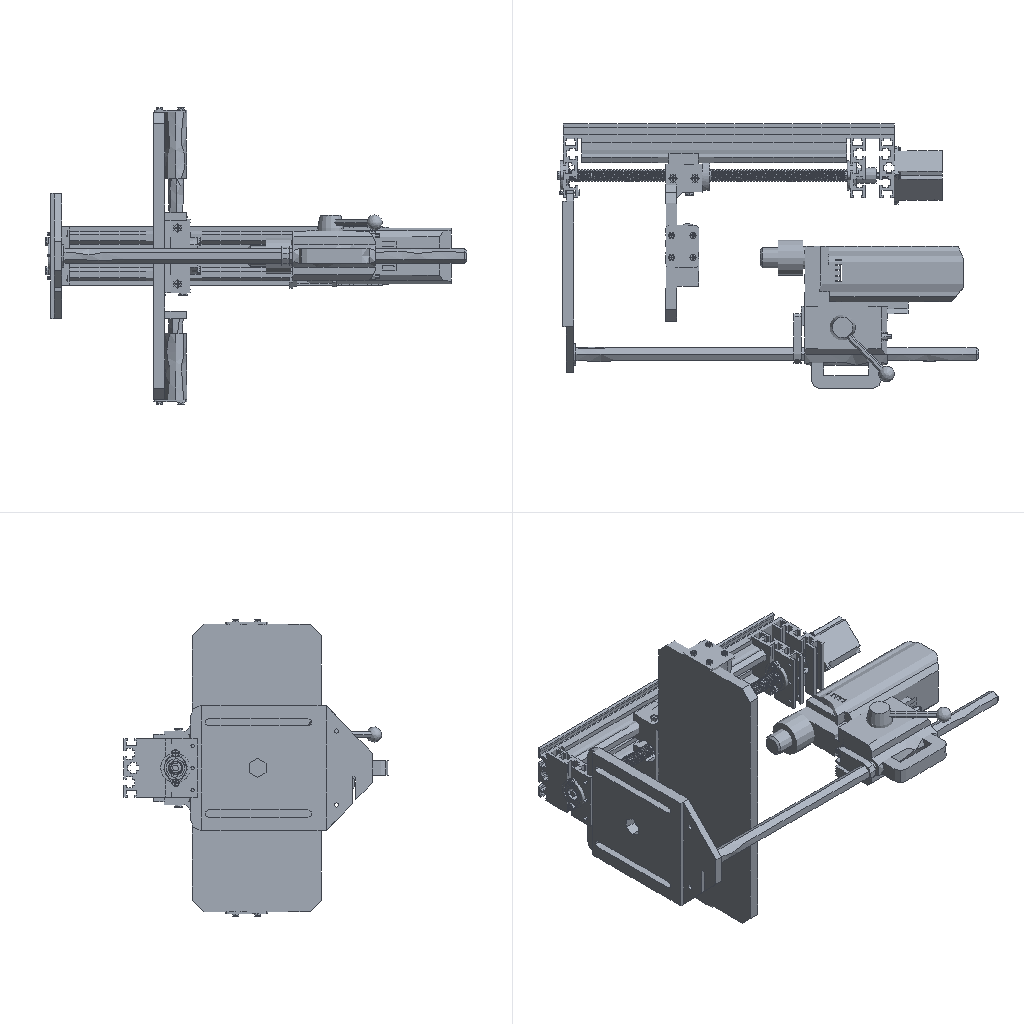Simulation study | ansys workbench
Set-up summary:
category,name,step,type,value,unit,region
solver,ansys_workbench
units,mm-N-s-tonne (MPa),,stated,"/units,MPA"
analysis,LS1,,static
load_step,LS1,LS1,static,nsubst=1; time=1
mesh,nodes,,,176175
mesh,elements,,,123008
element_type,SOLID187,,,82523
element_type,TARGE170,,,19068
element_type,CONTA174,,,19068
element_type,SOLID186,,,1937
element_type,SURF154,,,412
material,Structural Steel,,E,200000,tonne s^-2 mm^-1
material,Structural Steel,,nu,0.3
material,Structural Steel,,density,7.85e-09,tonne mm^-3
material,Structural Steel,,conductivity,60.5,tonne mm s^-3 C^-1
material,Structural Steel,,specific_heat,4.34e+08,mm^2 s^-2 C^-1
material,Structural Steel,,cte,1.2e-05,C^-1
material,Structural Steel,,permeability,10000
material,Structural Steel,,resistivity,0.00017,ohm mm
load,Define Force Using Surface Effect Elements,LS1,surface-effect pres face 1,-0.05982,,SURF154 #299
load,Define Force Using Surface Effect Elements,LS1,surface-effect pres face 3,-0.1976,,SURF154 #300
load,Define Force Using Surface Effect Elements,LS1,surface-effect pres face 3,0.1976,,SURF154 #301
bc,Fixed Supports,model,fixed,[dofs=ALL],,_FIXEDSU
contact,Contact Region,,bonded (always),element=CONTA174
contact,Contact Region 2,,bonded (always),element=CONTA174
contact,Contact Region 3,,bonded (always),element=CONTA174
contact,Contact Region 4,,bonded (always),element=CONTA174
contact,Contact Region 5,,bonded (always),element=CONTA174
contact,Contact Region 6,,bonded (always),element=CONTA174
contact,Contact Region 7,,bonded (always),element=CONTA174
contact,Contact Region 8,,bonded (always),element=CONTA174
contact,Contact Region 9,,bonded (always),element=CONTA174
contact,Contact Region 10,,bonded (always),element=CONTA174
contact,Contact Region 11,,bonded (always),element=CONTA174
contact,Contact Region 12,,bonded (always),element=CONTA174
contact,Contact Region 13,,bonded (always),element=CONTA174
contact,Contact Region 14,,bonded (always),element=CONTA174
contact,Contact Region 15,,bonded (always),element=CONTA174
contact,Contact Region 16,,bonded (always),element=CONTA174
contact,Contact Region 17,,bonded (always),element=CONTA174
contact,Contact Region 18,,bonded (always),element=CONTA174
contact,Contact Region 19,,bonded (always),element=CONTA174
contact,Contact Region 20,,bonded (always),element=CONTA174
contact,Contact Region 21,,bonded (always),element=CONTA174
contact,Contact Region 22,,bonded (always),element=CONTA174
contact,Contact Region 23,,bonded (always),element=CONTA174
contact,Contact Region 24,,bonded (always),element=CONTA174
contact,Contact Region 25,,bonded (always),element=CONTA174
contact,Contact Region 26,,bonded (always),element=CONTA174
contact,Contact Region 27,,bonded (always),element=CONTA174
contact,Contact Region 28,,bonded (always),element=CONTA174
contact,Contact Region 29,,bonded (always),element=CONTA174
contact,Contact Region 30,,bonded (always),element=CONTA174
contact,Contact Region 31,,bonded (always),element=CONTA174
contact,Contact Region 32,,bonded (always),element=CONTA174
contact,Contact Region 33,,bonded (always),element=CONTA174
contact,Contact Region 34,,bonded (always),element=CONTA174
contact,Contact Region 35,,bonded (always),element=CONTA174
contact,Contact Region 36,,bonded (always),element=CONTA174
contact,Contact Region 37,,bonded (always),element=CONTA174
contact,Contact Region 38,,bonded (always),element=CONTA174
contact,Contact Region 39,,bonded (always),element=CONTA174
contact,Contact Region 40,,bonded (always),element=CONTA174
contact,Contact Region 41,,bonded (always),element=CONTA174
contact,Contact Region 42,,bonded (always),element=CONTA174
contact,Contact Region 43,,bonded (always),element=CONTA174
contact,Contact Region 44,,bonded (always),element=CONTA174
contact,Contact Region 45,,bonded (always),element=CONTA174
contact,Contact Region 46,,bonded (always),element=CONTA174
contact,Contact Region 47,,bonded (always),element=CONTA174
contact,Contact Region 48,,bonded (always),element=CONTA174
contact,Contact Region 49,,bonded (always),element=CONTA174
contact,Contact Region 50,,bonded (always),element=CONTA174
contact,Contact Region 51,,bonded (always),element=CONTA174
contact,Contact Region 52,,bonded (always),element=CONTA174
contact,Contact Region 53,,bonded (always),element=CONTA174
contact,Contact Region 54,,bonded (always),element=CONTA174
contact,Contact Region 55,,bonded (always),element=CONTA174
contact,Contact Region 56,,bonded (always),element=CONTA174
contact,Contact Region 57,,bonded (always),element=CONTA174
contact,Contact Region 58,,bonded (always),element=CONTA174
contact,Contact Region 59,,bonded (always),element=CONTA174
contact,Contact Region 60,,bonded (always),element=CONTA174
contact,Contact Region 61,,bonded (always),element=CONTA174
contact,Contact Region 62,,bonded (always),element=CONTA174
contact,Contact Region 63,,bonded (always),element=CONTA174
contact,Contact Region 64,,bonded (always),element=CONTA174
contact,Contact Region 65,,bonded (always),element=CONTA174
contact,Contact Region 66,,bonded (always),element=CONTA174
contact,Contact Region 67,,bonded (always),element=CONTA174
contact,Contact Region 68,,bonded (always),element=CONTA174
contact,Contact Region 69,,bonded (always),element=CONTA174
contact,Contact Region 70,,bonded (always),element=CONTA174
contact,Contact Region 71,,bonded (always),element=CONTA174
contact,Contact Region 72,,bonded (always),element=CONTA174
contact,Contact Region 73,,bonded (always),element=CONTA174
contact,Contact Region 74,,bonded (always),element=CONTA174
contact,Contact Region 75,,bonded (always),element=CONTA174
contact,Contact Region 76,,bonded (always),element=CONTA174
contact,Contact Region 77,,bonded (always),element=CONTA174
contact,Contact Region 78,,bonded (always),element=CONTA174
contact,Contact Region 79,,bonded (always),element=CONTA174
contact,Contact Region 80,,bonded (always),element=CONTA174
contact,Contact Region 81,,bonded (always),element=CONTA174
contact,Contact Region 82,,bonded (always),element=CONTA174
contact,Contact Region 83,,bonded (always),element=CONTA174
contact,Contact Region 84,,bonded (always),element=CONTA174
contact,Contact Region 85,,bonded (always),element=CONTA174
contact,Contact Region 86,,bonded (always),element=CONTA174
contact,Contact Region 87,,bonded (always),element=CONTA174
contact,Contact Region 88,,bonded (always),element=CONTA174
contact,Contact Region 89,,bonded (always),element=CONTA174
contact,Contact Region 90,,bonded (always),element=CONTA174
contact,Contact Region 91,,bonded (always),element=CONTA174
contact,Contact Region 92,,bonded (always),element=CONTA174
contact,Contact Region 93,,bonded (always),element=CONTA174
contact,Contact Region 94,,bonded (always),element=CONTA174
contact,Contact Region 95,,bonded (always),element=CONTA174
contact,Contact Region 96,,bonded (always),element=CONTA174
contact,Contact Region 97,,bonded (always),element=CONTA174
contact,Contact Region 98,,bonded (always),element=CONTA174
contact,Contact Region 99,,bonded (always),element=CONTA174
contact,Contact Region 100,,bonded (always),element=CONTA174
contact,Contact Region 101,,bonded (always),element=CONTA174
contact,Contact Region 102,,bonded (always),element=CONTA174
contact,Contact Region 103,,bonded (always),element=CONTA174
contact,Contact Region 104,,bonded (always),element=CONTA174
contact,Contact Region 105,,bonded (always),element=CONTA174
contact,Contact Region 106,,bonded (always),element=CONTA174
contact,Contact Region 107,,bonded (always),element=CONTA174
contact,Contact Region 108,,bonded (always),element=CONTA174
contact,Contact Region 109,,bonded (always),element=CONTA174
contact,Contact Region 110,,bonded (always),element=CONTA174
contact,Contact Region 111,,bonded (always),element=CONTA174
contact,Contact Region 112,,bonded (always),element=CONTA174
named_set,_FIXEDSU,,node,69000
Ansys APDL input file, long lists of numbers shortened:
/batch
/config,noeldb,1     ! force off writing results to database
*get,_wallstrt,active,,time,wall
! ANSYS input file written by Workbench version 2022 R1
! File used for geometry attach:
/title,wbnew--____ (B5)
! ****** Begin Custom Load Command Snippet ******
/COM, ACT Extensions:
/COM,     LSDYNA, 2021.1
/COM,
! ****** End   Custom Load Command Snippet ******
*DIM,_wb_ProjectScratch_dir,string,248
_wb_ProjectScratch_dir(1) = ''
*DIM,_wb_SolverFiles_dir,string,248
_wb_SolverFiles_dir(1) = ''
*DIM,_wb_userfiles_dir,string,248
_wb_userfiles_dir(1) = ''
/com,--- Data in consistent NMM units. See Solving Units in the help system for more information.
/units,MPA
/nopr
/wb,file,start              !  signify a WB generated input file
/prep7
! Turn off shape checking because checks already performed inside WB mesher.
! See help system for more information.
SHPP,OFF,,NOWARN
/nolist
etcon,set             ! allow ANSYS to choose best KEYOP's for 180x elements, resets any applicable keyopt to MAPDL defaults
/com,*********** Nodes for the whole assembly ***********
nblock,3,,193792
(1i9,3e20.9e3)
        1     4.544231993E+01    -1.675656162E+02     8.308123616E-01
! (176174 more lines like these left out)
-1
/wb,elem,start            !  set before creation of elements
/com,*********** Elements for Body 1 "____|__-__3" ***********
et,1,187
eblock,19,solid,,10209
(19i9)
        1        1        1        1        0        0        0        0       10        0    47846    97468   101014    97470    97469   101844   101853   101839   101838
! (20417 more lines like these left out)
-1
/com,*********** Elements for Body 2 "____|__-__5" ***********
et,2,187
eblock,19,solid,,2459
(19i9)
        2        2        2        2        0        0        0        0       10        0    60222   123346   123792   124169   124165   124991   127779   124995   124994
! (4917 more lines like these left out)
-1
/com,*********** Elements for Body 3 "____|__-__5[2]" ***********
et,3,187
eblock,19,solid,,2459
(19i9)
        3        3        3        3        0        0        0        0       10        0    64453   133020   133466   133843   133839   134665   137453   134669   134668
! (4917 more lines like these left out)
-1
/com,*********** Elements for Body 4 "____ 2|__-__5" ***********
et,4,187
eblock,19,solid,,1587
(19i9)
        4        4        4        4        0        0        0        0       10        0    67164   139805   140360   139811   139812   140972   140997   140969   140970
! (3173 more lines like these left out)
-1
/com,*********** Elements for Body 5 "_______|__-__4" ***********
et,5,186
keyo,5,2,1          ! set full integration on SOLID186
eblock,19,solid,,252
(19i9)
        5        5        5        5        0        0        0        0       20        0    62681   128549   128760   128786   128558   128688   128746   128773   128679
! (503 more lines like these left out)
-1
! (69 more sections like these left out)
/wb,elem,end               !  done creating elements
/com,*********** Send User Defined Coordinate System(s) ***********
csys,0
toffst,273.15,  ! Temperature offset from absolute zero
/com,*********** Set Reference Temperature ***********
tref,22.
/wb,mat,start              !  starting to send materials
/com,*********** Send Materials ***********
Temperature = 'TEMP' ! Temperature
MP,DENS,1,7.85e-09,	! tonne mm^-3
MP,ALPX,1,1.2e-05,	! C^-1
MP,C,1,434000000,	! mm^2 s^-2 C^-1
MP,KXX,1,60.5,	! tonne mm s^-3 C^-1
MP,RSVX,1,0.00017,	! ohm mm
MP,EX,1,200000,	! tonne s^-2 mm^-1
MP,NUXY,1,0.3,
MP,MURX,1,10000,
Temperature = 'TEMP' ! Temperature
MP,DENS,2,7.85e-09,	! tonne mm^-3
MP,ALPX,2,1.2e-05,	! C^-1
MP,C,2,434000000,	! mm^2 s^-2 C^-1
MP,KXX,2,60.5,	! tonne mm s^-3 C^-1
MP,RSVX,2,0.00017,	! ohm mm
MP,EX,2,200000,	! tonne s^-2 mm^-1
MP,NUXY,2,0.3,
MP,MURX,2,10000,
Temperature = 'TEMP' ! Temperature
MP,DENS,3,7.85e-09,	! tonne mm^-3
MP,ALPX,3,1.2e-05,	! C^-1
MP,C,3,434000000,	! mm^2 s^-2 C^-1
MP,KXX,3,60.5,	! tonne mm s^-3 C^-1
MP,RSVX,3,0.00017,	! ohm mm
MP,EX,3,200000,	! tonne s^-2 mm^-1
MP,NUXY,3,0.3,
MP,MURX,3,10000,
Temperature = 'TEMP' ! Temperature
MP,DENS,4,7.85e-09,	! tonne mm^-3
MP,ALPX,4,1.2e-05,	! C^-1
MP,C,4,434000000,	! mm^2 s^-2 C^-1
MP,KXX,4,60.5,	! tonne mm s^-3 C^-1
MP,RSVX,4,0.00017,	! ohm mm
MP,EX,4,200000,	! tonne s^-2 mm^-1
MP,NUXY,4,0.3,
MP,MURX,4,10000,
Temperature = 'TEMP' ! Temperature
MP,DENS,5,7.85e-09,	! tonne mm^-3
MP,ALPX,5,1.2e-05,	! C^-1
MP,C,5,434000000,	! mm^2 s^-2 C^-1
MP,KXX,5,60.5,	! tonne mm s^-3 C^-1
MP,RSVX,5,0.00017,	! ohm mm
MP,EX,5,200000,	! tonne s^-2 mm^-1
MP,NUXY,5,0.3,
MP,MURX,5,10000,
Temperature = 'TEMP' ! Temperature
MP,DENS,6,7.85e-09,	! tonne mm^-3
MP,ALPX,6,1.2e-05,	! C^-1
MP,C,6,434000000,	! mm^2 s^-2 C^-1
MP,KXX,6,60.5,	! tonne mm s^-3 C^-1
MP,RSVX,6,0.00017,	! ohm mm
MP,EX,6,200000,	! tonne s^-2 mm^-1
MP,NUXY,6,0.3,
MP,MURX,6,10000,
Temperature = 'TEMP' ! Temperature
MP,DENS,7,7.85e-09,	! tonne mm^-3
MP,ALPX,7,1.2e-05,	! C^-1
MP,C,7,434000000,	! mm^2 s^-2 C^-1
MP,KXX,7,60.5,	! tonne mm s^-3 C^-1
MP,RSVX,7,0.00017,	! ohm mm
MP,EX,7,200000,	! tonne s^-2 mm^-1
MP,NUXY,7,0.3,
MP,MURX,7,10000,
Temperature = 'TEMP' ! Temperature
MP,DENS,8,7.85e-09,	! tonne mm^-3
MP,ALPX,8,1.2e-05,	! C^-1
MP,C,8,434000000,	! mm^2 s^-2 C^-1
MP,KXX,8,60.5,	! tonne mm s^-3 C^-1
MP,RSVX,8,0.00017,	! ohm mm
MP,EX,8,200000,	! tonne s^-2 mm^-1
MP,NUXY,8,0.3,
MP,MURX,8,10000,
Temperature = 'TEMP' ! Temperature
MP,DENS,9,7.85e-09,	! tonne mm^-3
MP,ALPX,9,1.2e-05,	! C^-1
MP,C,9,434000000,	! mm^2 s^-2 C^-1
MP,KXX,9,60.5,	! tonne mm s^-3 C^-1
MP,RSVX,9,0.00017,	! ohm mm
MP,EX,9,200000,	! tonne s^-2 mm^-1
! (587 more lines like these left out)
/wb,mat,end                !  done sending materials
!************************* Model Summary ********************
!____|__-__3,	结构钢,	matid,	1
!____|__-__5,	结构钢,	matid,	2
!____|__-__5[2],	结构钢,	matid,	3
! (73 more lines like these left out)
*get,_xmin,node,,mnloc,x
*get,_ymin,node,,mnloc,y
*get,_zmin,node,,mnloc,z
*get,_xmax,node,,mxloc,x
*get,_ymax,node,,mxloc,y
*get,_zmax,node,,mxloc,z
_ASMDIAG=(_xmax-_xmin)*(_xmax-_xmin)+(_ymax-_ymin)*(_ymax-_ymin)+(_zmax-_zmin)*(_zmax-_zmin)
_ASMDIAG=SQRT(_ASMDIAG)
/wb,contact,start          !  starting to send contact
/com,*********** Create Contact "接触区域" ***********
/com,            Real Constant Set For Above Contact Is 76 & 75
*set,tid,76
*set,cid,75
r,tid
r,cid
et,tid,170
et,cid,174
eblock,10,,,25
(15i9)
   137019       76       76       76        0    98298    98375   100949   100949   108146   108592   100949   108150
! (24 more lines like these left out)
-1
eblock,10,,,25
(15i9)
   137044       75       75       75        0    98298    98375   100949   100949   108146   108592   100949   108150
! (24 more lines like these left out)
-1
eblock,10,,,36
(15i9)
   137069       75       76       75        0   123537   123888   123538   123538   126120   126132   123538   126114
! (35 more lines like these left out)
-1
eblock,10,,,36
(15i9)
   137105       76       75       76        0   123537   123888   123538   123538   126120   126132   123538   126114
! (35 more lines like these left out)
-1
keyo,cid,8,2               ! auto create asymmetric contact (from Program Controlled setting)
keyo,cid,10,0              ! adjust contact stiffness each NR iteration (from Program Controlled setting)
keyo,cid,12,5              ! bonded always
keyo,cid,18,1              ! small sliding turned on by application
keyo,cid,2,0               ! augmented Lagrange (from Program Controlled setting)
keyo,cid,4,0               ! on Gauss point (from Program Controlled setting)
keyo,cid,9,1               ! ignore initial gaps/penetration
keyo,cid,7,0               ! No Prediction
rmod,tid,3,10.      ! FKN
rmod,tid,5,0.       ! ICONT
rmod,tid,6,0.       ! PINB
rmod,tid,10,0.      ! CNOF
rmod,tid,12,0.      ! FKT
rmod,tid,36,245     ! WB DSID
rmod,cid,3,10.      ! FKN
rmod,cid,5,0.       ! ICONT
rmod,cid,6,0.       ! PINB
rmod,cid,10,0.      ! CNOF
rmod,cid,12,0.      ! FKT
rmod,cid,36,245     ! WB DSID
/com,*********** Create Contact "接触区域 2" ***********
/com,            Real Constant Set For Above Contact Is 78 & 77
*set,tid,78
*set,cid,77
r,tid
r,cid
et,tid,170
et,cid,174
eblock,10,,,29
(15i9)
   137141       78       78       78        0    97360   100962    98362    98362   101192   108485    98362   101186
! (28 more lines like these left out)
-1
eblock,10,,,29
(15i9)
   137170       77       77       77        0    97360   100962    98362    98362   101192   108485    98362   101186
! (28 more lines like these left out)
-1
eblock,10,,,36
(15i9)
   137199       77       78       77        0   133211   133562   133212   133212   135794   135806   133212   135788
! (35 more lines like these left out)
-1
eblock,10,,,36
(15i9)
   137235       78       77       78        0   133211   133562   133212   133212   135794   135806   133212   135788
! (35 more lines like these left out)
-1
keyo,cid,8,2               ! auto create asymmetric contact (from Program Controlled setting)
keyo,cid,10,0              ! adjust contact stiffness each NR iteration (from Program Controlled setting)
keyo,cid,12,5              ! bonded always
keyo,cid,18,1              ! small sliding turned on by application
keyo,cid,2,0               ! augmented Lagrange (from Program Controlled setting)
keyo,cid,4,0               ! on Gauss point (from Program Controlled setting)
keyo,cid,9,1               ! ignore initial gaps/penetration
keyo,cid,7,0               ! No Prediction
rmod,tid,3,10.      ! FKN
rmod,tid,5,0.       ! ICONT
rmod,tid,6,0.       ! PINB
rmod,tid,10,0.      ! CNOF
rmod,tid,12,0.      ! FKT
rmod,tid,36,248     ! WB DSID
rmod,cid,3,10.      ! FKN
rmod,cid,5,0.       ! ICONT
rmod,cid,6,0.       ! PINB
rmod,cid,10,0.      ! CNOF
rmod,cid,12,0.      ! FKT
rmod,cid,36,248     ! WB DSID
/com,*********** Create Contact "接触区域 3" ***********
/com,            Real Constant Set For Above Contact Is 80 & 79
*set,tid,80
*set,cid,79
r,tid
r,cid
et,tid,170
et,cid,174
eblock,10,,,24
(15i9)
   137271       80       80       80        0    97359   100964   100963   100963   101181   118526   100963   101180
! (23 more lines like these left out)
-1
eblock,10,,,24
(15i9)
   137295       79       79       79        0    97359   100964   100963   100963   101181   118526   100963   101180
! (23 more lines like these left out)
-1
eblock,10,,,36
(15i9)
   137319       79       80       79        0   139961   140199   139962   139962   141831   141843   139962   141825
! (35 more lines like these left out)
-1
eblock,10,,,36
(15i9)
   137355       80       79       80        0   139961   140199   139962   139962   141831   141843   139962   141825
! (35 more lines like these left out)
-1
keyo,cid,8,2               ! auto create asymmetric contact (from Program Controlled setting)
keyo,cid,10,0              ! adjust contact stiffness each NR iteration (from Program Controlled setting)
keyo,cid,12,5              ! bonded always
keyo,cid,18,1              ! small sliding turned on by application
keyo,cid,2,0               ! augmented Lagrange (from Program Controlled setting)
keyo,cid,4,0               ! on Gauss point (from Program Controlled setting)
keyo,cid,9,1               ! ignore initial gaps/penetration
keyo,cid,7,0               ! No Prediction
rmod,tid,3,10.      ! FKN
rmod,tid,5,0.       ! ICONT
rmod,tid,6,0.       ! PINB
rmod,tid,10,0.      ! CNOF
rmod,tid,12,0.      ! FKT
rmod,tid,36,251     ! WB DSID
rmod,cid,3,10.      ! FKN
rmod,cid,5,0.       ! ICONT
rmod,cid,6,0.       ! PINB
rmod,cid,10,0.      ! CNOF
rmod,cid,12,0.      ! FKT
rmod,cid,36,251     ! WB DSID
/com,*********** Create Contact "接触区域 4" ***********
/com,            Real Constant Set For Above Contact Is 82 & 81
*set,tid,82
*set,cid,81
r,tid
r,cid
et,tid,170
et,cid,174
eblock,10,,,135
(15i9)
   137391       82       82       82        0    97368   100954    98370    98370   101299   108550    98370   101292
! (134 more lines like these left out)
-1
eblock,10,,,135
(15i9)
   137526       81       81       81        0    97368   100954    98370    98370   101299   108550    98370   101292
! (134 more lines like these left out)
-1
eblock,10,,,70
(15i9)
   137661       81       82       81        0   128702   128871   128856   128707   129495   129847   129506   129493
! (69 more lines like these left out)
-1
eblock,10,,,70
(15i9)
   137731       82       81       82        0   128702   128871   128856   128707   129495   129847   129506   129493
! (69 more lines like these left out)
-1
keyo,cid,8,2               ! auto create asymmetric contact (from Program Controlled setting)
keyo,cid,10,0              ! adjust contact stiffness each NR iteration (from Program Controlled setting)
keyo,cid,12,5              ! bonded always
keyo,cid,18,1              ! small sliding turned on by application
keyo,cid,2,0               ! augmented Lagrange (from Program Controlled setting)
keyo,cid,4,0               ! on Gauss point (from Program Controlled setting)
keyo,cid,9,1               ! ignore initial gaps/penetration
keyo,cid,7,0               ! No Prediction
rmod,tid,3,10.      ! FKN
rmod,tid,5,0.       ! ICONT
rmod,tid,6,0.       ! PINB
rmod,tid,10,0.      ! CNOF
rmod,tid,12,0.      ! FKT
rmod,tid,36,254     ! WB DSID
rmod,cid,3,10.      ! FKN
rmod,cid,5,0.       ! ICONT
rmod,cid,6,0.       ! PINB
rmod,cid,10,0.      ! CNOF
rmod,cid,12,0.      ! FKT
rmod,cid,36,254     ! WB DSID
/com,*********** Create Contact "接触区域 5" ***********
/com,            Real Constant Set For Above Contact Is 84 & 83
*set,tid,84
*set,cid,83
r,tid
r,cid
et,tid,170
et,cid,174
eblock,10,,,138
(15i9)
   137801       84       84       84        0    97598   100881    98506    98506   102979   109709    98506   102974
! (137 more lines like these left out)
-1
eblock,10,,,138
(15i9)
   137939       83       83       83        0    97598   100881    98506    98506   102979   109709    98506   102974
! (137 more lines like these left out)
-1
eblock,10,,,70
(15i9)
   138077       83       84       83        0   138376   138545   138530   138381   139169   139521   139180   139167
! (69 more lines like these left out)
-1
eblock,10,,,70
(15i9)
   138147       84       83       84        0   138376   138545   138530   138381   139169   139521   139180   139167
! (69 more lines like these left out)
-1
keyo,cid,8,2               ! auto create asymmetric contact (from Program Controlled setting)
keyo,cid,10,0              ! adjust contact stiffness each NR iteration (from Program Controlled setting)
keyo,cid,12,5              ! bonded always
keyo,cid,18,1              ! small sliding turned on by application
keyo,cid,2,0               ! augmented Lagrange (from Program Controlled setting)
keyo,cid,4,0               ! on Gauss point (from Program Controlled setting)
keyo,cid,9,1               ! ignore initial gaps/penetration
keyo,cid,7,0               ! No Prediction
rmod,tid,3,10.      ! FKN
rmod,tid,5,0.       ! ICONT
rmod,tid,6,0.       ! PINB
rmod,tid,10,0.      ! CNOF
rmod,tid,12,0.      ! FKT
rmod,tid,36,257     ! WB DSID
rmod,cid,3,10.      ! FKN
rmod,cid,5,0.       ! ICONT
rmod,cid,6,0.       ! PINB
rmod,cid,10,0.      ! CNOF
rmod,cid,12,0.      ! FKT
rmod,cid,36,257     ! WB DSID
! (107 more sections like these left out)
/wb,contact,end            !  done creating contacts
/golist
/wb,load,start             !  starting to send loads
/com,*********** Fixed Supports ***********
CMBLOCK,_FIXEDSU,NODE,    69000
(8i10)
        96        97        98        99       100       101       102       103
! (8624 more lines like these left out)
cmsel,s,_FIXEDSU
d,all,all
nsel,all
/com,*********** Define Force Using Surface Effect Elements ***********
local,12,0,0.,0.,0.,0.,0.,0.
csys,0
et,299,154
eblock,10,,,314
(15i9)
   175155      299      299      299       12   138421   138391   138417   138418   139199   139198   139261   139263
! (313 more lines like these left out)
-1
esel,s,type,,299
keyop,299,2,1                ! Apply load in local coordinate system
keyop,299,7,1                ! Use original area so load is constant in large deformation
esel,all
/com,*********** Define Force Using Surface Effect Elements ***********
local,13,0,0.,0.,0.,0.,0.,0.
csys,0
et,300,154
eblock,10,,,49
(15i9)
   175469      300      300      300       13    31080    31157    31082    31082    31244    31258    31082    31242
! (48 more lines like these left out)
-1
esel,s,type,,300
keyop,300,2,1                ! Apply load in local coordinate system
keyop,300,7,1                ! Use original area so load is constant in large deformation
esel,all
/com,*********** Define Force Using Surface Effect Elements ***********
local,14,0,0.,0.,0.,0.,0.,0.
csys,0
et,301,154
eblock,10,,,49
(15i9)
   175518      301      301      301       14    29252    29329    29254    29254    29416    29430    29254    29414
! (48 more lines like these left out)
-1
esel,s,type,,301
keyop,301,2,1                ! Apply load in local coordinate system
keyop,301,7,1                ! Use original area so load is constant in large deformation
esel,all
/gst,on,on
fini
*get,_numnode,node,0,count
*get,_numelem,elem,0,count
*get, _MAXELEMNUM, elem, 0, NUM, MAX
*get, _MAXNODENUM, node, 0, NUM, MAX
*get, _MAXELEMTYPE, etyp, 0, NUM, MAX
*get, _MAXREALCONST, real, 0, NUM, MAX
/go
/wb,load,end               !  done creating loads
/com,--- Number of total nodes = %_numnode%
/com,--- Number of contact elements = 38548
/com,--- Number of spring elements = 0
/com,--- Number of bearing elements = 0
/com,--- Number of solid elements = 84460
/com,--- Number of condensed parts = 0
/com,--- Number of total elements = %_numelem%
*get,_wallbsol,active,,time,wall
/com,****************************************************************************
/com,*************************    SOLUTION       ********************************
/com,****************************************************************************
/solu
antype,0                   ! static analysis
_thickRatio=0.486   ! Ratio of thick parts in the model
eqsl,sparse,,,,,1
cntr,print,1               ! print out contact info and also make no initial contact an error
cntr,out,yes               ! write contact output to file.cmn due to many contact pairs present
dmpoption,emat,no             ! Don't combine emat file for DANSYS
dmpoption,esav,no             ! Don't combine esav file for DANSYS
nldiag,cont,iter           ! print out contact info each equilibrium iteration
rescontrol,,none                 ! Do not keep any restart files
/com,****************************************************
/com,******************* SOLVE FOR LS 1 OF 1 ****************
esel,s,type,,299
nsle
sfe,all,1,pres,1,-5.98163568622454e-002
sfe,all,2,pres,1,0.
sfe,all,3,pres,1,0.
esel,s,type,,300
nsle
sfe,all,1,pres,1,0.
sfe,all,2,pres,1,0.
sfe,all,3,pres,1,-0.1976
esel,s,type,,301
nsle
sfe,all,1,pres,1,0.
sfe,all,2,pres,1,0.
sfe,all,3,pres,1,0.1976
nsel,all
esel,all
/nopr
/gopr
nsub,1,1,1
time,1.
outres,erase
outres,all,none
outres,nsol,all,
outres,rsol,all
outres,eangl,all
outres,etmp,all
outres,veng,all
outres,strs,all,
outres,epel,all,
outres,eppl,all,
outres,cont,all,
! *********** WB SOLVE COMMAND ***********
! check interactive state
*get,ANSINTER_,active,,int
*if,ANSINTER_,ne,0,then
/eof
*endif
solve
/com *************** Write FE CONNECTORS *********
CEWRITE,file,ce,,INTE
/com,****************************************************
/com,*************** FINISHED SOLVE FOR LS 1 *************
*get,_wallasol,active,,time,wall
/nopr
*get,_numnode,node,0,count
*get,_numelem,elem,0,count
*get, _MAXELEMNUM, elem, 0, NUM, MAX
*get, _MAXNODENUM, node, 0, NUM, MAX,,,INTERNAL
*get, _MAXELEMTYPE, etyp, 0, NUM, MAX
*get, _MAXREALCONST, real, 0, NUM, MAX
/gopr
/post1
xmlo,ENCODING,ISO-8859-1
xmlo,parm
/xml,parm,xml
fini
/gopr
*get,_walldone,active,,time,wall
_preptime=(_wallbsol-_wallstrt)*3600
_solvtime=(_wallasol-_wallbsol)*3600
_posttime=(_walldone-_wallasol)*3600
_totaltim=(_walldone-_wallstrt)*3600
*get,_dlbratio,active,0,solu,dlbr
*get,_combtime,active,0,solu,comb
*get,_ssmode,active,0,solu,ssmm
*get,_ndofs,active,0,solu,ndof
*get,_sol_end_time,active,0,set,time
*if,_sol_end_time,eq,1.,then
/fclean				!clean distributed files
*endif
/com,--- Total number of nodes = %_numnode%
/com,--- Total number of elements = %_numelem%
/com,--- Element load balance ratio = %_dlbratio%
/com,--- Time to combine distributed files = %_combtime%
/com,--- Sparse memory mode = %_ssmode%
/com,--- Number of DOF = %_ndofs%
/wb,file,end               ! done with WB generated input
Results summary:
result,analyses[0].index,,,1
result,analyses[0].system,,,SYS
result,analyses[0].deck,,,deck.dat
result,analyses[0].solve_status,,,completed
result,analyses[0].analysis_type,,,static
result,analyses[0].physics,,,mechanical
result,analyses[0].unit_system,,,"NMM: mm, ton, N, s, mV, mA, degC"
result,analyses[0].n_sets,,,1
result,analyses[0].load_steps[0].set,set=1,,1
result,analyses[0].load_steps[0].time_or_freq,set=1,,1
result,analyses[0].load_steps[0].max_displacement_magnitude,set=1,,0.004952
result,analyses[0].load_steps[0].max_von_mises_nodal,set=1,,8.774
result,analyses[0].load_steps[0].reaction_force_sum_xyz[1],set=1,,5000
result,analyses[0].load_steps[0].reaction_force_sum_xyz[2],set=1,,-0.0002834
result,analyses[0].load_steps[0].reaction_force_sum_xyz[3],set=1,,-7.56547e-05